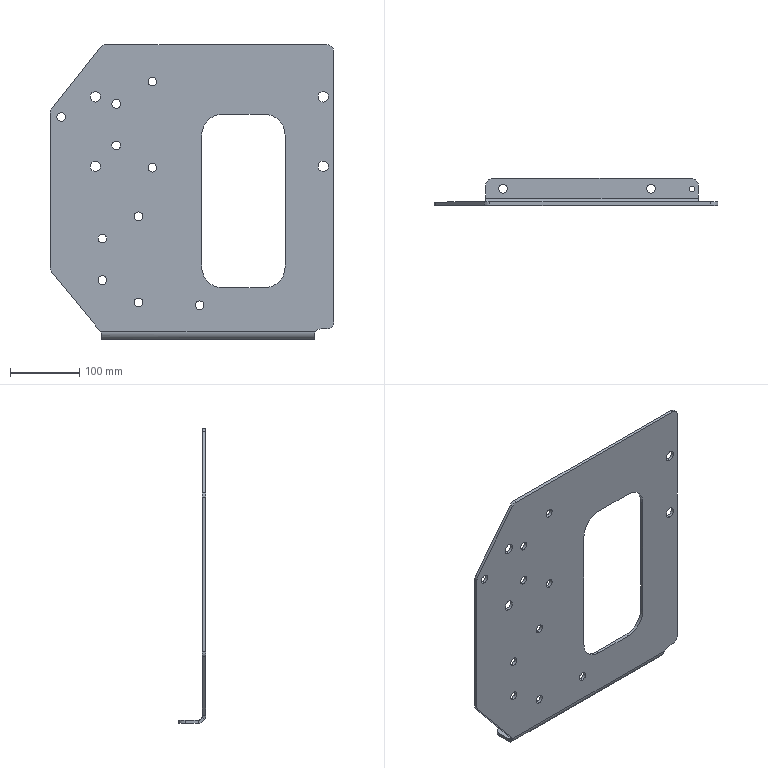Part | SolidWorks | features ICE 3, Fillet 1, FlatPattern 1, SMBaseFlange 1, SheetMetal 1 | 1 solid | 70 faces | box 408 x 39 x 424 mm | volume 643319 mm3 | cylinder 49 | plane 19 | spline 2 | commonest cylinder face diameters 12.5 x24 20 x9 15 x8 60 x4 8 x2 12 x1